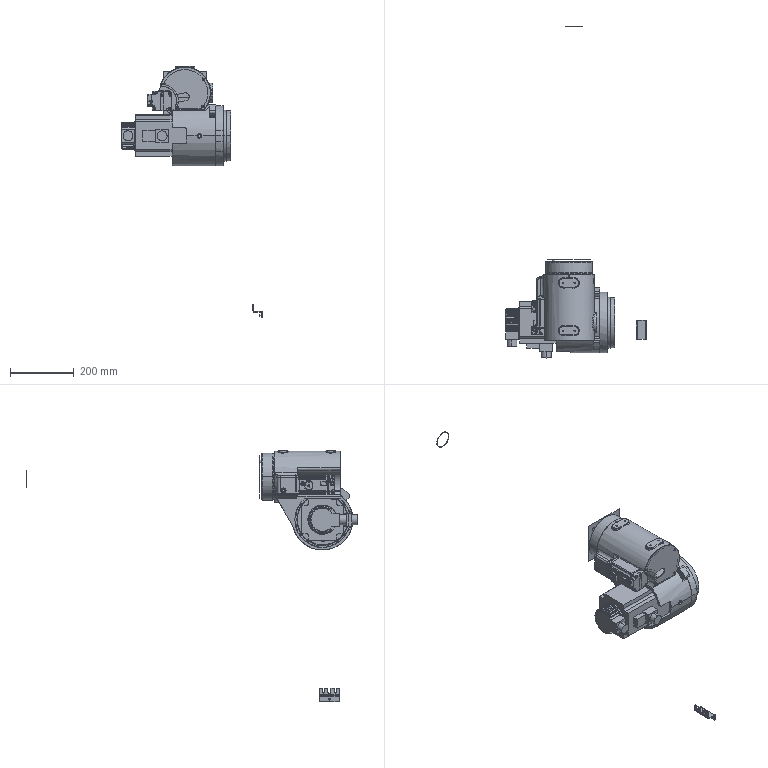Part | NX | features BREP 41 | 1 solid | 644 faces | box 441.537 x 1041 x 787.037 mm | volume 2214010 mm3 | cylinder 334 | plane 214 | torus 49 | spline 38 | cone 8 | sphere 1 | commonest cylinder face diameters 3 x43 1 x42 10 x30 4 x26 9 x26 6 x19